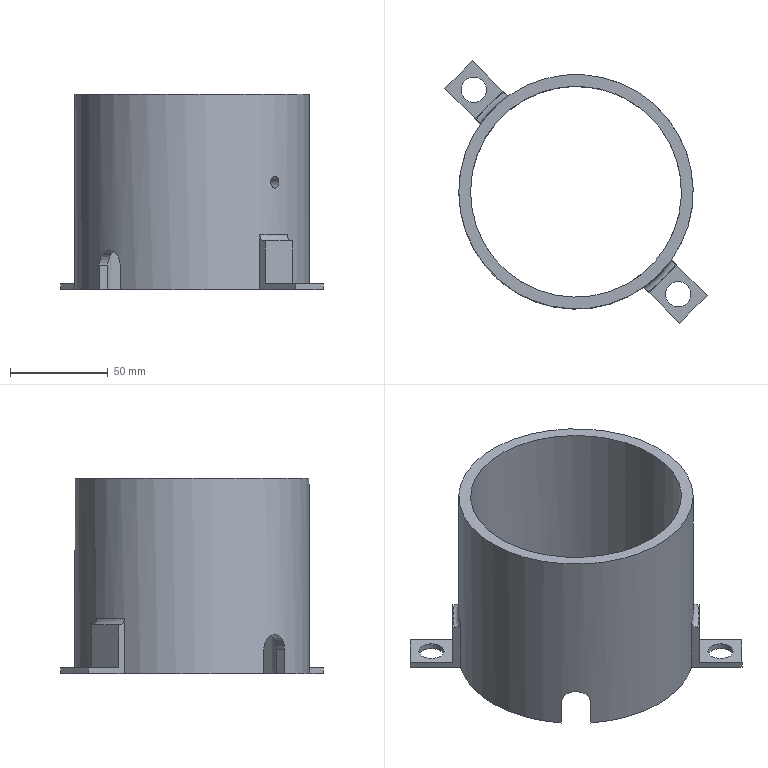Part | NX | features solid 2 | 1 solid | 30 faces | box 134.35 x 134.35 x 100 mm | volume 216597 mm3 | plane 21 | cylinder 7 | torus 2 | commonest cylinder face diameters 13 x2 15 x2 6 x1 108 x1 120 x1
STEP:
#1=CARTESIAN_POINT('',(1067.73,-417.73,-105.));
#2=VERTEX_POINT('',#1);
#3=CARTESIAN_POINT('',(1072.326,-422.326,-105.));
#4=DIRECTION('',(0.,0.,-1.));
#5=DIRECTION('',(-0.7071,0.7071,0.));
#6=AXIS2_PLACEMENT_3D('',#3,#4,#5);
#7=CIRCLE('',#6,6.5);
#8=EDGE_CURVE('',#2,#2,#7,.T.);
#9=ORIENTED_EDGE('',*,*,#8,.F.);
#10=EDGE_LOOP('',(#9));
#11=FACE_BOUND('',#10,.T.);
#12=CARTESIAN_POINT('',(1067.397,-333.21,-105.));
#13=VERTEX_POINT('',#12);
#14=CARTESIAN_POINT('',(1068.904,-404.762,-105.));
#15=VERTEX_POINT('',#14);
#16=CARTESIAN_POINT('',(1020.,-370.,-105.));
#17=DIRECTION('',(0.,0.,-1.));
#18=DIRECTION('',(-0.7071,0.7071,0.));
#19=AXIS2_PLACEMENT_3D('',#16,#17,#18);
#20=CIRCLE('',#19,60.);
#21=EDGE_CURVE('',#13,#15,#20,.T.);
#22=ORIENTED_EDGE('',*,*,#21,.T.);
#23=CARTESIAN_POINT('',(1087.175,-423.033,-105.));
#24=VERTEX_POINT('',#23);
#25=CARTESIAN_POINT('',(1065.255,-401.113,-105.));
#26=DIRECTION('',(0.7071,-0.7071,0.));
#27=VECTOR('',#26,1000.);
#28=LINE('',#25,#27);
#29=EDGE_CURVE('',#15,#24,#28,.T.);
#30=ORIENTED_EDGE('',*,*,#29,.T.);
#31=CARTESIAN_POINT('',(1073.033,-437.175,-105.));
#32=VERTEX_POINT('',#31);
#33=CARTESIAN_POINT('',(1073.033,-437.175,-105.));
#34=DIRECTION('',(0.7071,0.7071,0.));
#35=VECTOR('',#34,1000.);
#36=LINE('',#33,#35);
#37=EDGE_CURVE('',#32,#24,#36,.T.);
#38=ORIENTED_EDGE('',*,*,#37,.F.);
#39=CARTESIAN_POINT('',(1054.762,-418.904,-105.));
#40=VERTEX_POINT('',#39);
#41=CARTESIAN_POINT('',(1057.477,-421.619,-105.));
#42=DIRECTION('',(-0.7071,0.7071,0.));
#43=VECTOR('',#42,1000.);
#44=LINE('',#41,#43);
#45=EDGE_CURVE('',#32,#40,#44,.T.);
#46=ORIENTED_EDGE('',*,*,#45,.T.);
#47=CARTESIAN_POINT('',(983.21,-417.397,-105.));
#48=VERTEX_POINT('',#47);
#49=CARTESIAN_POINT('',(1020.,-370.,-105.));
#50=DIRECTION('',(0.,0.,-1.));
#51=DIRECTION('',(-0.7071,0.7071,0.));
#52=AXIS2_PLACEMENT_3D('',#49,#50,#51);
#53=CIRCLE('',#52,60.);
#54=EDGE_CURVE('',#40,#48,#53,.T.);
#55=ORIENTED_EDGE('',*,*,#54,.T.);
#56=CARTESIAN_POINT('',(987.49,-413.117,-105.));
#57=VERTEX_POINT('',#56);
#58=CARTESIAN_POINT('',(1025.303,-375.303,-105.));
#59=DIRECTION('',(-0.7071,-0.7071,0.));
#60=VECTOR('',#59,1000.);
#61=LINE('',#58,#60);
#62=EDGE_CURVE('',#57,#48,#61,.T.);
#63=ORIENTED_EDGE('',*,*,#62,.F.);
#64=CARTESIAN_POINT('',(1063.117,-337.49,-105.));
#65=VERTEX_POINT('',#64);
#66=CARTESIAN_POINT('',(1020.,-370.,-105.));
#67=DIRECTION('',(0.,0.,-1.));
#68=DIRECTION('',(-0.7071,0.7071,0.));
#69=AXIS2_PLACEMENT_3D('',#66,#67,#68);
#70=CIRCLE('',#69,54.);
#71=EDGE_CURVE('',#65,#57,#70,.T.);
#72=ORIENTED_EDGE('',*,*,#71,.F.);
#73=CARTESIAN_POINT('',(1025.303,-375.303,-105.));
#74=DIRECTION('',(-0.7071,-0.7071,0.));
#75=VECTOR('',#74,1000.);
#76=LINE('',#73,#75);
#77=EDGE_CURVE('',#13,#65,#76,.T.);
#78=ORIENTED_EDGE('',*,*,#77,.F.);
#79=EDGE_LOOP('',(#22,#30,#38,#46,#55,#63,#72,#78));
#80=FACE_BOUND('',#79,.T.);
#81=CARTESIAN_POINT('',(1020.,-370.,-105.));
#82=DIRECTION('',(0.,0.,1.));
#83=DIRECTION('',(-0.7071,0.7071,0.));
#84=AXIS2_PLACEMENT_3D('',#81,#82,#83);
#85=PLANE('',#84);
#86=ADVANCED_FACE('',(#11,#80),#85,.F.);
#87=CARTESIAN_POINT('',(982.523,-318.381,-80.));
#88=VERTEX_POINT('',#87);
#89=CARTESIAN_POINT('',(983.088,-318.946,-80.));
#90=VERTEX_POINT('',#89);
#91=CARTESIAN_POINT('',(982.523,-318.381,-80.));
#92=DIRECTION('',(0.7071,-0.7071,0.));
#93=VECTOR('',#92,1000.);
#94=LINE('',#91,#93);
#95=EDGE_CURVE('',#88,#90,#94,.T.);
#96=ORIENTED_EDGE('',*,*,#95,.F.);
#97=CARTESIAN_POINT('',(975.452,-325.452,-80.));
#98=VERTEX_POINT('',#97);
#99=CARTESIAN_POINT('',(968.381,-332.523,-80.));
#100=DIRECTION('',(0.7071,0.7071,0.));
#101=VECTOR('',#100,1000.);
#102=LINE('',#99,#101);
#103=EDGE_CURVE('',#98,#88,#102,.T.);
#104=ORIENTED_EDGE('',*,*,#103,.F.);
#105=CARTESIAN_POINT('',(1020.,-370.,-80.));
#106=DIRECTION('',(0.,0.,-1.));
#107=DIRECTION('',(-0.7071,0.7071,0.));
#108=AXIS2_PLACEMENT_3D('',#105,#106,#107);
#109=CIRCLE('',#108,63.);
#110=EDGE_CURVE('',#90,#98,#109,.F.);
#111=ORIENTED_EDGE('',*,*,#110,.F.);
#112=EDGE_LOOP('',(#96,#104,#111));
#113=FACE_BOUND('',#112,.T.);
#114=CARTESIAN_POINT('',(988.887,-324.745,-80.));
#115=DIRECTION('',(0.,0.,1.));
#116=DIRECTION('',(-0.7071,0.7071,0.));
#117=AXIS2_PLACEMENT_3D('',#114,#115,#116);
#118=PLANE('',#117);
#119=ADVANCED_FACE('',(#113),#118,.T.);
#120=CARTESIAN_POINT('',(1057.477,-421.619,-80.));
#121=VERTEX_POINT('',#120);
#122=CARTESIAN_POINT('',(1056.912,-421.054,-80.));
#123=VERTEX_POINT('',#122);
#124=CARTESIAN_POINT('',(1057.477,-421.619,-80.));
#125=DIRECTION('',(-0.7071,0.7071,0.));
#126=VECTOR('',#125,1000.);
#127=LINE('',#124,#126);
#128=EDGE_CURVE('',#121,#123,#127,.T.);
#129=ORIENTED_EDGE('',*,*,#128,.F.);
#130=CARTESIAN_POINT('',(1064.548,-414.548,-80.));
#131=VERTEX_POINT('',#130);
#132=CARTESIAN_POINT('',(1071.619,-407.477,-80.));
#133=DIRECTION('',(-0.7071,-0.7071,0.));
#134=VECTOR('',#133,1000.);
#135=LINE('',#132,#134);
#136=EDGE_CURVE('',#131,#121,#135,.T.);
#137=ORIENTED_EDGE('',*,*,#136,.F.);
#138=CARTESIAN_POINT('',(1020.,-370.,-80.));
#139=DIRECTION('',(0.,0.,-1.));
#140=DIRECTION('',(-0.7071,0.7071,0.));
#141=AXIS2_PLACEMENT_3D('',#138,#139,#140);
#142=CIRCLE('',#141,63.);
#143=EDGE_CURVE('',#123,#131,#142,.F.);
#144=ORIENTED_EDGE('',*,*,#143,.F.);
#145=EDGE_LOOP('',(#129,#137,#144));
#146=FACE_BOUND('',#145,.T.);
#147=CARTESIAN_POINT('',(1057.477,-421.619,-80.));
#148=DIRECTION('',(0.,0.,1.));
#149=DIRECTION('',(-0.7071,0.7071,0.));
#150=AXIS2_PLACEMENT_3D('',#147,#148,#149);
#151=PLANE('',#150);
#152=ADVANCED_FACE('',(#146),#151,.T.);
#153=CARTESIAN_POINT('',(1062.426,-412.426,-47.));
#154=VERTEX_POINT('',#153);
#155=CARTESIAN_POINT('',(1064.064,-410.736,-47.651));
#156=CARTESIAN_POINT('',(1062.439,-412.44,-46.675));
#157=CARTESIAN_POINT('',(1060.737,-414.062,-47.65));
#158=CARTESIAN_POINT('',(1060.01,-414.711,-49.998));
#159=CARTESIAN_POINT('',(1060.736,-414.063,-52.35));
#160=CARTESIAN_POINT('',(1062.439,-412.44,-53.324));
#161=CARTESIAN_POINT('',(1064.06,-410.74,-52.353));
#162=CARTESIAN_POINT('',(1064.711,-410.009,-50.003));
#163=CARTESIAN_POINT('',(1064.064,-410.736,-47.651));
#164=CARTESIAN_POINT('',(1062.439,-412.44,-46.675));
#165=CARTESIAN_POINT('',(1060.737,-414.062,-47.65));
#166=B_SPLINE_CURVE_WITH_KNOTS('',3,(#155,#156,#157,#158,#159,#160,#161,#162,#163,#164,#165),.UNSPECIFIED.,.T.,.F.,(1,1,1,1,1,1,1,1,1,1,1,1,1,1,1),(-0.007035,-0.00469,-0.002345,0.,0.002345,0.00469,0.007035,0.00938,0.01172,0.01407,0.01641,0.01876,0.0211,0.02345,0.02579),.UNSPECIFIED.);
#167=EDGE_CURVE('',#154,#154,#166,.T.);
#168=ORIENTED_EDGE('',*,*,#167,.F.);
#169=EDGE_LOOP('',(#168));
#170=FACE_BOUND('',#169,.T.);
#171=CARTESIAN_POINT('',(960.,-370.,-5.));
#172=VERTEX_POINT('',#171);
#173=CARTESIAN_POINT('',(1020.,-370.,-5.));
#174=DIRECTION('',(0.,0.,-1.));
#175=DIRECTION('',(-1.,0.,0.));
#176=AXIS2_PLACEMENT_3D('',#173,#174,#175);
#177=CIRCLE('',#176,60.);
#178=EDGE_CURVE('',#172,#172,#177,.T.);
#179=ORIENTED_EDGE('',*,*,#178,.T.);
#180=EDGE_LOOP('',(#179));
#181=FACE_BOUND('',#180,.T.);
#182=CARTESIAN_POINT('',(1056.79,-322.603,-92.5));
#183=VERTEX_POINT('',#182);
#184=CARTESIAN_POINT('',(1067.397,-333.21,-92.5));
#185=VERTEX_POINT('',#184);
#186=CARTESIAN_POINT('',(1056.79,-322.603,-92.5));
#187=CARTESIAN_POINT('',(1056.79,-322.603,-90.541));
#188=CARTESIAN_POINT('',(1058.106,-323.584,-86.621));
#189=CARTESIAN_POINT('',(1062.512,-327.494,-84.187));
#190=CARTESIAN_POINT('',(1066.415,-331.893,-86.633));
#191=CARTESIAN_POINT('',(1067.397,-333.21,-90.516));
#192=CARTESIAN_POINT('',(1067.397,-333.21,-92.5));
#193=B_SPLINE_CURVE_WITH_KNOTS('',3,(#186,#187,#188,#189,#190,#191,#192),.UNSPECIFIED.,.F.,.F.,(4,1,1,1,4),(0.01174,0.01761,0.02347,0.02934,0.03521),.UNSPECIFIED.);
#194=EDGE_CURVE('',#183,#185,#193,.T.);
#195=ORIENTED_EDGE('',*,*,#194,.F.);
#196=CARTESIAN_POINT('',(1056.79,-322.603,-105.));
#197=VERTEX_POINT('',#196);
#198=CARTESIAN_POINT('',(1056.79,-322.603,5.));
#199=DIRECTION('',(0.,0.,-1.));
#200=VECTOR('',#199,1000.);
#201=LINE('',#198,#200);
#202=EDGE_CURVE('',#197,#183,#201,.F.);
#203=ORIENTED_EDGE('',*,*,#202,.F.);
#204=CARTESIAN_POINT('',(985.238,-321.096,-105.));
#205=VERTEX_POINT('',#204);
#206=CARTESIAN_POINT('',(1020.,-370.,-105.));
#207=DIRECTION('',(0.,0.,-1.));
#208=DIRECTION('',(-0.7071,0.7071,0.));
#209=AXIS2_PLACEMENT_3D('',#206,#207,#208);
#210=CIRCLE('',#209,60.);
#211=EDGE_CURVE('',#205,#197,#210,.T.);
#212=ORIENTED_EDGE('',*,*,#211,.F.);
#213=CARTESIAN_POINT('',(985.238,-321.096,-77.));
#214=VERTEX_POINT('',#213);
#215=CARTESIAN_POINT('',(985.238,-321.096,5.));
#216=DIRECTION('',(0.,0.,-1.));
#217=VECTOR('',#216,1000.);
#218=LINE('',#215,#217);
#219=EDGE_CURVE('',#205,#214,#218,.F.);
#220=ORIENTED_EDGE('',*,*,#219,.T.);
#221=CARTESIAN_POINT('',(971.096,-335.238,-77.));
#222=VERTEX_POINT('',#221);
#223=CARTESIAN_POINT('',(1020.,-370.,-77.));
#224=DIRECTION('',(0.,0.,-1.));
#225=DIRECTION('',(-0.7071,0.7071,0.));
#226=AXIS2_PLACEMENT_3D('',#223,#224,#225);
#227=CIRCLE('',#226,60.);
#228=EDGE_CURVE('',#222,#214,#227,.T.);
#229=ORIENTED_EDGE('',*,*,#228,.F.);
#230=CARTESIAN_POINT('',(971.096,-335.238,-105.));
#231=VERTEX_POINT('',#230);
#232=CARTESIAN_POINT('',(971.096,-335.238,5.));
#233=DIRECTION('',(0.,0.,-1.));
#234=VECTOR('',#233,1000.);
#235=LINE('',#232,#234);
#236=EDGE_CURVE('',#222,#231,#235,.T.);
#237=ORIENTED_EDGE('',*,*,#236,.T.);
#238=CARTESIAN_POINT('',(972.603,-406.79,-105.));
#239=VERTEX_POINT('',#238);
#240=CARTESIAN_POINT('',(1020.,-370.,-105.));
#241=DIRECTION('',(0.,0.,-1.));
#242=DIRECTION('',(-0.7071,0.7071,0.));
#243=AXIS2_PLACEMENT_3D('',#240,#241,#242);
#244=CIRCLE('',#243,60.);
#245=EDGE_CURVE('',#239,#231,#244,.T.);
#246=ORIENTED_EDGE('',*,*,#245,.F.);
#247=CARTESIAN_POINT('',(972.603,-406.79,-92.5));
#248=VERTEX_POINT('',#247);
#249=CARTESIAN_POINT('',(972.603,-406.79,5.));
#250=DIRECTION('',(0.,0.,-1.));
#251=VECTOR('',#250,1000.);
#252=LINE('',#249,#251);
#253=EDGE_CURVE('',#248,#239,#252,.T.);
#254=ORIENTED_EDGE('',*,*,#253,.F.);
#255=CARTESIAN_POINT('',(983.21,-417.397,-92.5));
#256=VERTEX_POINT('',#255);
#257=CARTESIAN_POINT('',(983.21,-417.397,-92.5));
#258=CARTESIAN_POINT('',(983.21,-417.397,-90.517));
#259=CARTESIAN_POINT('',(981.896,-416.418,-86.634));
#260=CARTESIAN_POINT('',(977.485,-412.504,-84.184));
#261=CARTESIAN_POINT('',(973.581,-408.101,-86.631));
#262=CARTESIAN_POINT('',(972.603,-406.79,-90.542));
#263=CARTESIAN_POINT('',(972.603,-406.79,-92.5));
#264=B_SPLINE_CURVE_WITH_KNOTS('',3,(#257,#258,#259,#260,#261,#262,#263),.UNSPECIFIED.,.F.,.F.,(4,1,1,1,4),(0.03521,0.04108,0.04694,0.05281,0.05868),.UNSPECIFIED.);
#265=EDGE_CURVE('',#256,#248,#264,.T.);
#266=ORIENTED_EDGE('',*,*,#265,.F.);
#267=CARTESIAN_POINT('',(983.21,-417.397,5.));
#268=DIRECTION('',(0.,0.,-1.));
#269=VECTOR('',#268,1000.);
#270=LINE('',#267,#269);
#271=EDGE_CURVE('',#48,#256,#270,.F.);
#272=ORIENTED_EDGE('',*,*,#271,.F.);
#273=ORIENTED_EDGE('',*,*,#54,.F.);
#274=CARTESIAN_POINT('',(1054.762,-418.904,-77.));
#275=VERTEX_POINT('',#274);
#276=CARTESIAN_POINT('',(1054.762,-418.904,5.));
#277=DIRECTION('',(0.,0.,-1.));
#278=VECTOR('',#277,1000.);
#279=LINE('',#276,#278);
#280=EDGE_CURVE('',#40,#275,#279,.F.);
#281=ORIENTED_EDGE('',*,*,#280,.T.);
#282=CARTESIAN_POINT('',(1068.904,-404.762,-77.));
#283=VERTEX_POINT('',#282);
#284=CARTESIAN_POINT('',(1020.,-370.,-77.));
#285=DIRECTION('',(0.,0.,-1.));
#286=DIRECTION('',(-0.7071,0.7071,0.));
#287=AXIS2_PLACEMENT_3D('',#284,#285,#286);
#288=CIRCLE('',#287,60.);
#289=EDGE_CURVE('',#283,#275,#288,.T.);
#290=ORIENTED_EDGE('',*,*,#289,.F.);
#291=CARTESIAN_POINT('',(1068.904,-404.762,5.));
#292=DIRECTION('',(0.,0.,-1.));
#293=VECTOR('',#292,1000.);
#294=LINE('',#291,#293);
#295=EDGE_CURVE('',#283,#15,#294,.T.);
#296=ORIENTED_EDGE('',*,*,#295,.T.);
#297=ORIENTED_EDGE('',*,*,#21,.F.);
#298=CARTESIAN_POINT('',(1067.397,-333.21,5.));
#299=DIRECTION('',(0.,0.,-1.));
#300=VECTOR('',#299,1000.);
#301=LINE('',#298,#300);
#302=EDGE_CURVE('',#185,#13,#301,.T.);
#303=ORIENTED_EDGE('',*,*,#302,.F.);
#304=EDGE_LOOP('',(#195,#203,#212,#220,#229,#237,#246,#254,#266,#272,#273,#281,#290,#296,#297,#303));
#305=FACE_BOUND('',#304,.T.);
#306=CARTESIAN_POINT('',(1020.,-370.,5.));
#307=DIRECTION('',(0.,0.,-1.));
#308=DIRECTION('',(0.7071,-0.7071,0.));
#309=AXIS2_PLACEMENT_3D('',#306,#307,#308);
#310=CYLINDRICAL_SURFACE('',#309,60.);
#311=ADVANCED_FACE('',(#170,#181,#305),#310,.T.);
#312=CARTESIAN_POINT('',(1063.117,-337.49,-92.5));
#313=VERTEX_POINT('',#312);
#314=CARTESIAN_POINT('',(1063.117,-337.49,5.));
#315=DIRECTION('',(0.,0.,-1.));
#316=VECTOR('',#315,1000.);
#317=LINE('',#314,#316);
#318=EDGE_CURVE('',#313,#65,#317,.T.);
#319=ORIENTED_EDGE('',*,*,#318,.T.);
#320=ORIENTED_EDGE('',*,*,#71,.T.);
#321=CARTESIAN_POINT('',(987.49,-413.117,-92.5));
#322=VERTEX_POINT('',#321);
#323=CARTESIAN_POINT('',(987.49,-413.117,5.));
#324=DIRECTION('',(0.,0.,-1.));
#325=VECTOR('',#324,1000.);
#326=LINE('',#323,#325);
#327=EDGE_CURVE('',#57,#322,#326,.F.);
#328=ORIENTED_EDGE('',*,*,#327,.T.);
#329=CARTESIAN_POINT('',(976.883,-402.51,-92.5));
#330=VERTEX_POINT('',#329);
#331=CARTESIAN_POINT('',(987.49,-413.117,-92.5));
#332=CARTESIAN_POINT('',(987.49,-413.117,-90.517));
#333=CARTESIAN_POINT('',(986.158,-412.157,-86.634));
#334=CARTESIAN_POINT('',(981.719,-408.271,-84.184));
#335=CARTESIAN_POINT('',(977.842,-403.84,-86.631));
#336=CARTESIAN_POINT('',(976.883,-402.51,-90.541));
#337=CARTESIAN_POINT('',(976.883,-402.51,-92.5));
#338=B_SPLINE_CURVE_WITH_KNOTS('',3,(#331,#332,#333,#334,#335,#336,#337),.UNSPECIFIED.,.F.,.F.,(4,1,1,1,4),(0.03522,0.04109,0.04695,0.05282,0.05869),.UNSPECIFIED.);
#339=EDGE_CURVE('',#322,#330,#338,.T.);
#340=ORIENTED_EDGE('',*,*,#339,.T.);
#341=CARTESIAN_POINT('',(976.883,-402.51,-105.));
#342=VERTEX_POINT('',#341);
#343=CARTESIAN_POINT('',(976.883,-402.51,5.));
#344=DIRECTION('',(0.,0.,-1.));
#345=VECTOR('',#344,1000.);
#346=LINE('',#343,#345);
#347=EDGE_CURVE('',#330,#342,#346,.T.);
#348=ORIENTED_EDGE('',*,*,#347,.T.);
#349=CARTESIAN_POINT('',(1052.51,-326.883,-105.));
#350=VERTEX_POINT('',#349);
#351=CARTESIAN_POINT('',(1020.,-370.,-105.));
#352=DIRECTION('',(0.,0.,-1.));
#353=DIRECTION('',(-0.7071,0.7071,0.));
#354=AXIS2_PLACEMENT_3D('',#351,#352,#353);
#355=CIRCLE('',#354,54.);
#356=EDGE_CURVE('',#342,#350,#355,.T.);
#357=ORIENTED_EDGE('',*,*,#356,.T.);
#358=CARTESIAN_POINT('',(1052.51,-326.883,-92.5));
#359=VERTEX_POINT('',#358);
#360=CARTESIAN_POINT('',(1052.51,-326.883,5.));
#361=DIRECTION('',(0.,0.,-1.));
#362=VECTOR('',#361,1000.);
#363=LINE('',#360,#362);
#364=EDGE_CURVE('',#350,#359,#363,.F.);
#365=ORIENTED_EDGE('',*,*,#364,.T.);
#366=CARTESIAN_POINT('',(1052.51,-326.883,-92.5));
#367=CARTESIAN_POINT('',(1052.51,-326.883,-90.541));
#368=CARTESIAN_POINT('',(1053.845,-327.845,-86.621));
#369=CARTESIAN_POINT('',(1058.279,-331.727,-84.187));
#370=CARTESIAN_POINT('',(1062.154,-336.154,-86.632));
#371=CARTESIAN_POINT('',(1063.117,-337.49,-90.517));
#372=CARTESIAN_POINT('',(1063.117,-337.49,-92.5));
#373=B_SPLINE_CURVE_WITH_KNOTS('',3,(#366,#367,#368,#369,#370,#371,#372),.UNSPECIFIED.,.F.,.F.,(4,1,1,1,4),(0.01174,0.01761,0.02348,0.02935,0.03522),.UNSPECIFIED.);
#374=EDGE_CURVE('',#359,#313,#373,.T.);
#375=ORIENTED_EDGE('',*,*,#374,.T.);
#376=EDGE_LOOP('',(#319,#320,#328,#340,#348,#357,#365,#375));
#377=FACE_BOUND('',#376,.T.);
#378=CARTESIAN_POINT('',(1058.184,-408.184,-47.));
#379=VERTEX_POINT('',#378);
#380=CARTESIAN_POINT('',(1059.818,-406.49,-47.651));
#381=CARTESIAN_POINT('',(1058.198,-408.199,-46.675));
#382=CARTESIAN_POINT('',(1056.492,-409.817,-47.65));
#383=CARTESIAN_POINT('',(1055.76,-410.461,-49.998));
#384=CARTESIAN_POINT('',(1056.491,-409.818,-52.35));
#385=CARTESIAN_POINT('',(1058.198,-408.199,-53.324));
#386=CARTESIAN_POINT('',(1059.815,-406.494,-52.353));
#387=CARTESIAN_POINT('',(1060.461,-405.759,-50.003));
#388=CARTESIAN_POINT('',(1059.818,-406.49,-47.651));
#389=CARTESIAN_POINT('',(1058.198,-408.199,-46.675));
#390=CARTESIAN_POINT('',(1056.492,-409.817,-47.65));
#391=B_SPLINE_CURVE_WITH_KNOTS('',3,(#380,#381,#382,#383,#384,#385,#386,#387,#388,#389,#390),.UNSPECIFIED.,.T.,.F.,(1,1,1,1,1,1,1,1,1,1,1,1,1,1,1),(-0.007035,-0.00469,-0.002345,0.,0.002345,0.00469,0.007035,0.00938,0.01173,0.01407,0.01642,0.01876,0.02111,0.02345,0.0258),.UNSPECIFIED.);
#392=EDGE_CURVE('',#379,#379,#391,.T.);
#393=ORIENTED_EDGE('',*,*,#392,.T.);
#394=EDGE_LOOP('',(#393));
#395=FACE_BOUND('',#394,.T.);
#396=CARTESIAN_POINT('',(966.,-370.,-5.));
#397=VERTEX_POINT('',#396);
#398=CARTESIAN_POINT('',(1020.,-370.,-5.));
#399=DIRECTION('',(0.,0.,-1.));
#400=DIRECTION('',(-1.,0.,0.));
#401=AXIS2_PLACEMENT_3D('',#398,#399,#400);
#402=CIRCLE('',#401,54.);
#403=EDGE_CURVE('',#397,#397,#402,.T.);
#404=ORIENTED_EDGE('',*,*,#403,.F.);
#405=EDGE_LOOP('',(#404));
#406=FACE_BOUND('',#405,.T.);
#407=CARTESIAN_POINT('',(1020.,-370.,5.));
#408=DIRECTION('',(0.,0.,-1.));
#409=DIRECTION('',(0.7071,-0.7071,0.));
#410=AXIS2_PLACEMENT_3D('',#407,#408,#409);
#411=CYLINDRICAL_SURFACE('',#410,54.);
#412=ADVANCED_FACE('',(#377,#395,#406),#411,.F.);
#413=ORIENTED_EDGE('',*,*,#403,.T.);
#414=EDGE_LOOP('',(#413));
#415=FACE_BOUND('',#414,.T.);
#416=ORIENTED_EDGE('',*,*,#178,.F.);
#417=EDGE_LOOP('',(#416));
#418=FACE_BOUND('',#417,.T.);
#419=CARTESIAN_POINT('',(1020.,-370.,-5.));
#420=DIRECTION('',(0.,0.,1.));
#421=DIRECTION('',(-0.7071,0.7071,0.));
#422=AXIS2_PLACEMENT_3D('',#419,#420,#421);
#423=PLANE('',#422);
#424=ADVANCED_FACE('',(#415,#418),#423,.T.);
#425=ORIENTED_EDGE('',*,*,#356,.F.);
#426=CARTESIAN_POINT('',(1014.697,-364.697,-105.));
#427=DIRECTION('',(0.7071,0.7071,0.));
#428=VECTOR('',#427,1000.);
#429=LINE('',#426,#428);
#430=EDGE_CURVE('',#239,#342,#429,.T.);
#431=ORIENTED_EDGE('',*,*,#430,.F.);
#432=ORIENTED_EDGE('',*,*,#245,.T.);
#433=CARTESIAN_POINT('',(952.825,-316.967,-105.));
#434=VERTEX_POINT('',#433);
#435=CARTESIAN_POINT('',(974.745,-338.887,-105.));
#436=DIRECTION('',(-0.7071,0.7071,0.));
#437=VECTOR('',#436,1000.);
#438=LINE('',#435,#437);
#439=EDGE_CURVE('',#231,#434,#438,.T.);
#440=ORIENTED_EDGE('',*,*,#439,.T.);
#441=CARTESIAN_POINT('',(966.967,-302.825,-105.));
#442=VERTEX_POINT('',#441);
#443=CARTESIAN_POINT('',(966.967,-302.825,-105.));
#444=DIRECTION('',(-0.7071,-0.7071,0.));
#445=VECTOR('',#444,1000.);
#446=LINE('',#443,#445);
#447=EDGE_CURVE('',#442,#434,#446,.T.);
#448=ORIENTED_EDGE('',*,*,#447,.F.);
#449=CARTESIAN_POINT('',(982.523,-318.381,-105.));
#450=DIRECTION('',(0.7071,-0.7071,0.));
#451=VECTOR('',#450,1000.);
#452=LINE('',#449,#451);
#453=EDGE_CURVE('',#442,#205,#452,.T.);
#454=ORIENTED_EDGE('',*,*,#453,.T.);
#455=ORIENTED_EDGE('',*,*,#211,.T.);
#456=CARTESIAN_POINT('',(1014.697,-364.697,-105.));
#457=DIRECTION('',(0.7071,0.7071,0.));
#458=VECTOR('',#457,1000.);
#459=LINE('',#456,#458);
#460=EDGE_CURVE('',#350,#197,#459,.T.);
#461=ORIENTED_EDGE('',*,*,#460,.F.);
#462=EDGE_LOOP('',(#425,#431,#432,#440,#448,#454,#455,#461));
#463=FACE_BOUND('',#462,.T.);
#464=CARTESIAN_POINT('',(963.078,-313.078,-105.));
#465=VERTEX_POINT('',#464);
#466=CARTESIAN_POINT('',(967.674,-317.674,-105.));
#467=DIRECTION('',(0.,0.,-1.));
#468=DIRECTION('',(-0.7071,0.7071,0.));
#469=AXIS2_PLACEMENT_3D('',#466,#467,#468);
#470=CIRCLE('',#469,6.5);
#471=EDGE_CURVE('',#465,#465,#470,.T.);
#472=ORIENTED_EDGE('',*,*,#471,.F.);
#473=EDGE_LOOP('',(#472));
#474=FACE_BOUND('',#473,.T.);
#475=CARTESIAN_POINT('',(1020.,-370.,-105.));
#476=DIRECTION('',(0.,0.,1.));
#477=DIRECTION('',(-0.7071,0.7071,0.));
#478=AXIS2_PLACEMENT_3D('',#475,#476,#477);
#479=PLANE('',#478);
#480=ADVANCED_FACE('',(#463,#474),#479,.F.);
#481=CARTESIAN_POINT('',(1071.619,-407.477,-80.));
#482=VERTEX_POINT('',#481);
#483=CARTESIAN_POINT('',(1071.619,-407.477,-80.));
#484=DIRECTION('',(-0.7071,-0.7071,0.));
#485=VECTOR('',#484,1000.);
#486=LINE('',#483,#485);
#487=EDGE_CURVE('',#482,#131,#486,.T.);
#488=ORIENTED_EDGE('',*,*,#487,.F.);
#489=CARTESIAN_POINT('',(1071.054,-406.912,-80.));
#490=VERTEX_POINT('',#489);
#491=CARTESIAN_POINT('',(1065.255,-401.113,-80.));
#492=DIRECTION('',(0.7071,-0.7071,0.));
#493=VECTOR('',#492,1000.);
#494=LINE('',#491,#493);
#495=EDGE_CURVE('',#490,#482,#494,.T.);
#496=ORIENTED_EDGE('',*,*,#495,.F.);
#497=CARTESIAN_POINT('',(1020.,-370.,-80.));
#498=DIRECTION('',(0.,0.,-1.));
#499=DIRECTION('',(-0.7071,0.7071,0.));
#500=AXIS2_PLACEMENT_3D('',#497,#498,#499);
#501=CIRCLE('',#500,63.);
#502=EDGE_CURVE('',#131,#490,#501,.F.);
#503=ORIENTED_EDGE('',*,*,#502,.F.);
#504=EDGE_LOOP('',(#488,#496,#503));
#505=FACE_BOUND('',#504,.T.);
#506=CARTESIAN_POINT('',(1057.477,-421.619,-80.));
#507=DIRECTION('',(0.,0.,1.));
#508=DIRECTION('',(-0.7071,0.7071,0.));
#509=AXIS2_PLACEMENT_3D('',#506,#507,#508);
#510=PLANE('',#509);
#511=ADVANCED_FACE('',(#505),#510,.T.);
#512=ORIENTED_EDGE('',*,*,#45,.F.);
#513=CARTESIAN_POINT('',(1073.033,-437.175,-102.));
#514=VERTEX_POINT('',#513);
#515=CARTESIAN_POINT('',(1073.033,-437.175,-102.));
#516=DIRECTION('',(0.,0.,-1.));
#517=VECTOR('',#516,1000.);
#518=LINE('',#515,#517);
#519=EDGE_CURVE('',#514,#32,#518,.T.);
#520=ORIENTED_EDGE('',*,*,#519,.F.);
#521=CARTESIAN_POINT('',(1057.477,-421.619,-102.));
#522=VERTEX_POINT('',#521);
#523=CARTESIAN_POINT('',(1057.477,-421.619,-102.));
#524=DIRECTION('',(0.7071,-0.7071,0.));
#525=VECTOR('',#524,1000.);
#526=LINE('',#523,#525);
#527=EDGE_CURVE('',#522,#514,#526,.T.);
#528=ORIENTED_EDGE('',*,*,#527,.F.);
#529=CARTESIAN_POINT('',(1057.477,-421.619,-80.));
#530=DIRECTION('',(0.,0.,-1.));
#531=VECTOR('',#530,1000.);
#532=LINE('',#529,#531);
#533=EDGE_CURVE('',#121,#522,#532,.T.);
#534=ORIENTED_EDGE('',*,*,#533,.F.);
#535=ORIENTED_EDGE('',*,*,#128,.T.);
#536=CARTESIAN_POINT('',(1054.762,-418.904,-77.));
#537=CARTESIAN_POINT('',(1054.762,-418.904,-77.798));
#538=CARTESIAN_POINT('',(1055.238,-419.38,-79.356));
#539=CARTESIAN_POINT('',(1056.348,-420.49,-80.));
#540=CARTESIAN_POINT('',(1056.912,-421.054,-80.));
#541=B_SPLINE_CURVE_WITH_KNOTS('',3,(#536,#537,#538,#539,#540),.UNSPECIFIED.,.F.,.F.,(4,1,4),(0.,0.002359,0.004718),.UNSPECIFIED.);
#542=EDGE_CURVE('',#275,#123,#541,.T.);
#543=ORIENTED_EDGE('',*,*,#542,.F.);
#544=ORIENTED_EDGE('',*,*,#280,.F.);
#545=EDGE_LOOP('',(#512,#520,#528,#534,#535,#543,#544));
#546=FACE_BOUND('',#545,.T.);
#547=CARTESIAN_POINT('',(1057.477,-421.619,-80.));
#548=DIRECTION('',(0.7071,0.7071,0.));
#549=DIRECTION('',(0.7071,-0.7071,0.));
#550=AXIS2_PLACEMENT_3D('',#547,#548,#549);
#551=PLANE('',#550);
#552=ADVANCED_FACE('',(#546),#551,.F.);
#553=ORIENTED_EDGE('',*,*,#495,.T.);
#554=CARTESIAN_POINT('',(1071.619,-407.477,-102.));
#555=VERTEX_POINT('',#554);
#556=CARTESIAN_POINT('',(1071.619,-407.477,-80.));
#557=DIRECTION('',(0.,0.,-1.));
#558=VECTOR('',#557,1000.);
#559=LINE('',#556,#558);
#560=EDGE_CURVE('',#482,#555,#559,.T.);
#561=ORIENTED_EDGE('',*,*,#560,.T.);
#562=CARTESIAN_POINT('',(1087.175,-423.033,-102.));
#563=VERTEX_POINT('',#562);
#564=CARTESIAN_POINT('',(1087.175,-423.033,-102.));
#565=DIRECTION('',(-0.7071,0.7071,0.));
#566=VECTOR('',#565,1000.);
#567=LINE('',#564,#566);
#568=EDGE_CURVE('',#563,#555,#567,.T.);
#569=ORIENTED_EDGE('',*,*,#568,.F.);
#570=CARTESIAN_POINT('',(1087.175,-423.033,-102.));
#571=DIRECTION('',(0.,0.,-1.));
#572=VECTOR('',#571,1000.);
#573=LINE('',#570,#572);
#574=EDGE_CURVE('',#563,#24,#573,.T.);
#575=ORIENTED_EDGE('',*,*,#574,.T.);
#576=ORIENTED_EDGE('',*,*,#29,.F.);
#577=ORIENTED_EDGE('',*,*,#295,.F.);
#578=CARTESIAN_POINT('',(1071.054,-406.912,-80.));
#579=CARTESIAN_POINT('',(1070.49,-406.348,-80.));
#580=CARTESIAN_POINT('',(1069.382,-405.24,-79.359));
#581=CARTESIAN_POINT('',(1068.904,-404.762,-77.798));
#582=CARTESIAN_POINT('',(1068.904,-404.762,-77.));
#583=B_SPLINE_CURVE_WITH_KNOTS('',3,(#578,#579,#580,#581,#582),.UNSPECIFIED.,.F.,.F.,(4,1,4),(0.,0.002359,0.004718),.UNSPECIFIED.);
#584=EDGE_CURVE('',#490,#283,#583,.T.);
#585=ORIENTED_EDGE('',*,*,#584,.F.);
#586=EDGE_LOOP('',(#553,#561,#569,#575,#576,#577,#585));
#587=FACE_BOUND('',#586,.T.);
#588=CARTESIAN_POINT('',(1065.255,-401.113,-80.));
#589=DIRECTION('',(-0.7071,-0.7071,0.));
#590=DIRECTION('',(-0.7071,0.7071,0.));
#591=AXIS2_PLACEMENT_3D('',#588,#589,#590);
#592=PLANE('',#591);
#593=ADVANCED_FACE('',(#587),#592,.F.);
#594=ORIENTED_EDGE('',*,*,#560,.F.);
#595=ORIENTED_EDGE('',*,*,#487,.T.);
#596=ORIENTED_EDGE('',*,*,#136,.T.);
#597=ORIENTED_EDGE('',*,*,#533,.T.);
#598=CARTESIAN_POINT('',(1071.619,-407.477,-102.));
#599=DIRECTION('',(-0.7071,-0.7071,0.));
#600=VECTOR('',#599,1000.);
#601=LINE('',#598,#600);
#602=EDGE_CURVE('',#555,#522,#601,.T.);
#603=ORIENTED_EDGE('',*,*,#602,.F.);
#604=EDGE_LOOP('',(#594,#595,#596,#597,#603));
#605=FACE_BOUND('',#604,.T.);
#606=CARTESIAN_POINT('',(1071.619,-407.477,-80.));
#607=DIRECTION('',(-0.7071,0.7071,0.));
#608=DIRECTION('',(0.,0.,-1.));
#609=AXIS2_PLACEMENT_3D('',#606,#607,#608);
#610=PLANE('',#609);
#611=ADVANCED_FACE('',(#605),#610,.F.);
#612=CARTESIAN_POINT('',(968.381,-332.523,-80.));
#613=VERTEX_POINT('',#612);
#614=CARTESIAN_POINT('',(968.381,-332.523,-80.));
#615=DIRECTION('',(0.7071,0.7071,0.));
#616=VECTOR('',#615,1000.);
#617=LINE('',#614,#616);
#618=EDGE_CURVE('',#613,#98,#617,.T.);
#619=ORIENTED_EDGE('',*,*,#618,.F.);
#620=CARTESIAN_POINT('',(968.946,-333.088,-80.));
#621=VERTEX_POINT('',#620);
#622=CARTESIAN_POINT('',(974.745,-338.887,-80.));
#623=DIRECTION('',(-0.7071,0.7071,0.));
#624=VECTOR('',#623,1000.);
#625=LINE('',#622,#624);
#626=EDGE_CURVE('',#621,#613,#625,.T.);
#627=ORIENTED_EDGE('',*,*,#626,.F.);
#628=CARTESIAN_POINT('',(1020.,-370.,-80.));
#629=DIRECTION('',(0.,0.,-1.));
#630=DIRECTION('',(-0.7071,0.7071,0.));
#631=AXIS2_PLACEMENT_3D('',#628,#629,#630);
#632=CIRCLE('',#631,63.);
#633=EDGE_CURVE('',#98,#621,#632,.F.);
#634=ORIENTED_EDGE('',*,*,#633,.F.);
#635=EDGE_LOOP('',(#619,#627,#634));
#636=FACE_BOUND('',#635,.T.);
#637=CARTESIAN_POINT('',(988.887,-324.745,-80.));
#638=DIRECTION('',(0.,0.,1.));
#639=DIRECTION('',(-0.7071,0.7071,0.));
#640=AXIS2_PLACEMENT_3D('',#637,#638,#639);
#641=PLANE('',#640);
#642=ADVANCED_FACE('',(#636),#641,.T.);
#643=ORIENTED_EDGE('',*,*,#453,.F.);
#644=CARTESIAN_POINT('',(966.967,-302.825,-102.));
#645=VERTEX_POINT('',#644);
#646=CARTESIAN_POINT('',(966.967,-302.825,-102.));
#647=DIRECTION('',(0.,0.,-1.));
#648=VECTOR('',#647,1000.);
#649=LINE('',#646,#648);
#650=EDGE_CURVE('',#645,#442,#649,.T.);
#651=ORIENTED_EDGE('',*,*,#650,.F.);
#652=CARTESIAN_POINT('',(982.523,-318.381,-102.));
#653=VERTEX_POINT('',#652);
#654=CARTESIAN_POINT('',(982.523,-318.381,-102.));
#655=DIRECTION('',(-0.7071,0.7071,0.));
#656=VECTOR('',#655,1000.);
#657=LINE('',#654,#656);
#658=EDGE_CURVE('',#653,#645,#657,.T.);
#659=ORIENTED_EDGE('',*,*,#658,.F.);
#660=CARTESIAN_POINT('',(982.523,-318.381,-80.));
#661=DIRECTION('',(0.,0.,-1.));
#662=VECTOR('',#661,1000.);
#663=LINE('',#660,#662);
#664=EDGE_CURVE('',#88,#653,#663,.T.);
#665=ORIENTED_EDGE('',*,*,#664,.F.);
#666=ORIENTED_EDGE('',*,*,#95,.T.);
#667=CARTESIAN_POINT('',(985.238,-321.096,-77.));
#668=CARTESIAN_POINT('',(985.238,-321.096,-77.798));
#669=CARTESIAN_POINT('',(984.762,-320.62,-79.356));
#670=CARTESIAN_POINT('',(983.652,-319.51,-80.));
#671=CARTESIAN_POINT('',(983.088,-318.946,-80.));
#672=B_SPLINE_CURVE_WITH_KNOTS('',3,(#667,#668,#669,#670,#671),.UNSPECIFIED.,.F.,.F.,(4,1,4),(0.,0.002359,0.004718),.UNSPECIFIED.);
#673=EDGE_CURVE('',#214,#90,#672,.T.);
#674=ORIENTED_EDGE('',*,*,#673,.F.);
#675=ORIENTED_EDGE('',*,*,#219,.F.);
#676=EDGE_LOOP('',(#643,#651,#659,#665,#666,#674,#675));
#677=FACE_BOUND('',#676,.T.);
#678=CARTESIAN_POINT('',(982.523,-318.381,-80.));
#679=DIRECTION('',(-0.7071,-0.7071,0.));
#680=DIRECTION('',(-0.7071,0.7071,0.));
#681=AXIS2_PLACEMENT_3D('',#678,#679,#680);
#682=PLANE('',#681);
#683=ADVANCED_FACE('',(#677),#682,.F.);
#684=ORIENTED_EDGE('',*,*,#626,.T.);
#685=CARTESIAN_POINT('',(968.381,-332.523,-102.));
#686=VERTEX_POINT('',#685);
#687=CARTESIAN_POINT('',(968.381,-332.523,-80.));
#688=DIRECTION('',(0.,0.,-1.));
#689=VECTOR('',#688,1000.);
#690=LINE('',#687,#689);
#691=EDGE_CURVE('',#613,#686,#690,.T.);
#692=ORIENTED_EDGE('',*,*,#691,.T.);
#693=CARTESIAN_POINT('',(952.825,-316.967,-102.));
#694=VERTEX_POINT('',#693);
#695=CARTESIAN_POINT('',(952.825,-316.967,-102.));
#696=DIRECTION('',(0.7071,-0.7071,0.));
#697=VECTOR('',#696,1000.);
#698=LINE('',#695,#697);
#699=EDGE_CURVE('',#694,#686,#698,.T.);
#700=ORIENTED_EDGE('',*,*,#699,.F.);
#701=CARTESIAN_POINT('',(952.825,-316.967,-102.));
#702=DIRECTION('',(0.,0.,-1.));
#703=VECTOR('',#702,1000.);
#704=LINE('',#701,#703);
#705=EDGE_CURVE('',#694,#434,#704,.T.);
#706=ORIENTED_EDGE('',*,*,#705,.T.);
#707=ORIENTED_EDGE('',*,*,#439,.F.);
#708=ORIENTED_EDGE('',*,*,#236,.F.);
#709=CARTESIAN_POINT('',(968.946,-333.088,-80.));
#710=CARTESIAN_POINT('',(969.51,-333.652,-80.));
#711=CARTESIAN_POINT('',(970.618,-334.76,-79.359));
#712=CARTESIAN_POINT('',(971.096,-335.238,-77.798));
#713=CARTESIAN_POINT('',(971.096,-335.238,-77.));
#714=B_SPLINE_CURVE_WITH_KNOTS('',3,(#709,#710,#711,#712,#713),.UNSPECIFIED.,.F.,.F.,(4,1,4),(0.,0.002359,0.004718),.UNSPECIFIED.);
#715=EDGE_CURVE('',#621,#222,#714,.T.);
#716=ORIENTED_EDGE('',*,*,#715,.F.);
#717=EDGE_LOOP('',(#684,#692,#700,#706,#707,#708,#716));
#718=FACE_BOUND('',#717,.T.);
#719=CARTESIAN_POINT('',(974.745,-338.887,-80.));
#720=DIRECTION('',(0.7071,0.7071,0.));
#721=DIRECTION('',(0.,0.,1.));
#722=AXIS2_PLACEMENT_3D('',#719,#720,#721);
#723=PLANE('',#722);
#724=ADVANCED_FACE('',(#718),#723,.F.);
#725=ORIENTED_EDGE('',*,*,#691,.F.);
#726=ORIENTED_EDGE('',*,*,#618,.T.);
#727=ORIENTED_EDGE('',*,*,#103,.T.);
#728=ORIENTED_EDGE('',*,*,#664,.T.);
#729=CARTESIAN_POINT('',(968.381,-332.523,-102.));
#730=DIRECTION('',(0.7071,0.7071,0.));
#731=VECTOR('',#730,1000.);
#732=LINE('',#729,#731);
#733=EDGE_CURVE('',#686,#653,#732,.T.);
#734=ORIENTED_EDGE('',*,*,#733,.F.);
#735=EDGE_LOOP('',(#725,#726,#727,#728,#734));
#736=FACE_BOUND('',#735,.T.);
#737=CARTESIAN_POINT('',(968.381,-332.523,-80.));
#738=DIRECTION('',(0.7071,-0.7071,0.));
#739=DIRECTION('',(0.,0.,1.));
#740=AXIS2_PLACEMENT_3D('',#737,#738,#739);
#741=PLANE('',#740);
#742=ADVANCED_FACE('',(#736),#741,.F.);
#743=ORIENTED_EDGE('',*,*,#447,.T.);
#744=ORIENTED_EDGE('',*,*,#705,.F.);
#745=CARTESIAN_POINT('',(966.967,-302.825,-102.));
#746=DIRECTION('',(-0.7071,-0.7071,0.));
#747=VECTOR('',#746,1000.);
#748=LINE('',#745,#747);
#749=EDGE_CURVE('',#645,#694,#748,.T.);
#750=ORIENTED_EDGE('',*,*,#749,.F.);
#751=ORIENTED_EDGE('',*,*,#650,.T.);
#752=EDGE_LOOP('',(#743,#744,#750,#751));
#753=FACE_BOUND('',#752,.T.);
#754=CARTESIAN_POINT('',(966.967,-302.825,-102.));
#755=DIRECTION('',(-0.7071,0.7071,0.));
#756=DIRECTION('',(0.,0.,-1.));
#757=AXIS2_PLACEMENT_3D('',#754,#755,#756);
#758=PLANE('',#757);
#759=ADVANCED_FACE('',(#753),#758,.T.);
#760=CARTESIAN_POINT('',(963.078,-313.078,-102.));
#761=VERTEX_POINT('',#760);
#762=CARTESIAN_POINT('',(967.674,-317.674,-102.));
#763=DIRECTION('',(0.,0.,-1.));
#764=DIRECTION('',(-0.7071,0.7071,0.));
#765=AXIS2_PLACEMENT_3D('',#762,#763,#764);
#766=CIRCLE('',#765,6.5);
#767=EDGE_CURVE('',#761,#761,#766,.T.);
#768=ORIENTED_EDGE('',*,*,#767,.F.);
#769=EDGE_LOOP('',(#768));
#770=FACE_BOUND('',#769,.T.);
#771=ORIENTED_EDGE('',*,*,#471,.T.);
#772=EDGE_LOOP('',(#771));
#773=FACE_BOUND('',#772,.T.);
#774=CARTESIAN_POINT('',(967.674,-317.674,-102.));
#775=DIRECTION('',(0.,0.,-1.));
#776=DIRECTION('',(0.7071,-0.7071,0.));
#777=AXIS2_PLACEMENT_3D('',#774,#775,#776);
#778=CYLINDRICAL_SURFACE('',#777,6.5);
#779=ADVANCED_FACE('',(#770,#773),#778,.F.);
#780=ORIENTED_EDGE('',*,*,#749,.T.);
#781=ORIENTED_EDGE('',*,*,#699,.T.);
#782=ORIENTED_EDGE('',*,*,#733,.T.);
#783=ORIENTED_EDGE('',*,*,#658,.T.);
#784=EDGE_LOOP('',(#780,#781,#782,#783));
#785=FACE_BOUND('',#784,.T.);
#786=ORIENTED_EDGE('',*,*,#767,.T.);
#787=EDGE_LOOP('',(#786));
#788=FACE_BOUND('',#787,.T.);
#789=CARTESIAN_POINT('',(952.825,-316.967,-102.));
#790=DIRECTION('',(0.,0.,-1.));
#791=DIRECTION('',(0.7071,-0.7071,0.));
#792=AXIS2_PLACEMENT_3D('',#789,#790,#791);
#793=PLANE('',#792);
#794=ADVANCED_FACE('',(#785,#788),#793,.F.);
#795=ORIENTED_EDGE('',*,*,#37,.T.);
#796=ORIENTED_EDGE('',*,*,#574,.F.);
#797=CARTESIAN_POINT('',(1073.033,-437.175,-102.));
#798=DIRECTION('',(0.7071,0.7071,0.));
#799=VECTOR('',#798,1000.);
#800=LINE('',#797,#799);
#801=EDGE_CURVE('',#514,#563,#800,.T.);
#802=ORIENTED_EDGE('',*,*,#801,.F.);
#803=ORIENTED_EDGE('',*,*,#519,.T.);
#804=EDGE_LOOP('',(#795,#796,#802,#803));
#805=FACE_BOUND('',#804,.T.);
#806=CARTESIAN_POINT('',(1073.033,-437.175,-102.));
#807=DIRECTION('',(0.7071,-0.7071,0.));
#808=DIRECTION('',(0.,0.,1.));
#809=AXIS2_PLACEMENT_3D('',#806,#807,#808);
#810=PLANE('',#809);
#811=ADVANCED_FACE('',(#805),#810,.T.);
#812=CARTESIAN_POINT('',(1067.73,-417.73,-102.));
#813=VERTEX_POINT('',#812);
#814=CARTESIAN_POINT('',(1072.326,-422.326,-102.));
#815=DIRECTION('',(0.,0.,-1.));
#816=DIRECTION('',(-0.7071,0.7071,0.));
#817=AXIS2_PLACEMENT_3D('',#814,#815,#816);
#818=CIRCLE('',#817,6.5);
#819=EDGE_CURVE('',#813,#813,#818,.T.);
#820=ORIENTED_EDGE('',*,*,#819,.F.);
#821=EDGE_LOOP('',(#820));
#822=FACE_BOUND('',#821,.T.);
#823=ORIENTED_EDGE('',*,*,#8,.T.);
#824=EDGE_LOOP('',(#823));
#825=FACE_BOUND('',#824,.T.);
#826=CARTESIAN_POINT('',(1072.326,-422.326,-102.));
#827=DIRECTION('',(0.,0.,-1.));
#828=DIRECTION('',(0.7071,-0.7071,0.));
#829=AXIS2_PLACEMENT_3D('',#826,#827,#828);
#830=CYLINDRICAL_SURFACE('',#829,6.5);
#831=ADVANCED_FACE('',(#822,#825),#830,.F.);
#832=ORIENTED_EDGE('',*,*,#801,.T.);
#833=ORIENTED_EDGE('',*,*,#568,.T.);
#834=ORIENTED_EDGE('',*,*,#602,.T.);
#835=ORIENTED_EDGE('',*,*,#527,.T.);
#836=EDGE_LOOP('',(#832,#833,#834,#835));
#837=FACE_BOUND('',#836,.T.);
#838=ORIENTED_EDGE('',*,*,#819,.T.);
#839=EDGE_LOOP('',(#838));
#840=FACE_BOUND('',#839,.T.);
#841=CARTESIAN_POINT('',(1087.175,-423.033,-102.));
#842=DIRECTION('',(0.,0.,-1.));
#843=DIRECTION('',(0.7071,-0.7071,0.));
#844=AXIS2_PLACEMENT_3D('',#841,#842,#843);
#845=PLANE('',#844);
#846=ADVANCED_FACE('',(#837,#840),#845,.F.);
#847=ORIENTED_EDGE('',*,*,#502,.T.);
#848=ORIENTED_EDGE('',*,*,#584,.T.);
#849=ORIENTED_EDGE('',*,*,#289,.T.);
#850=ORIENTED_EDGE('',*,*,#542,.T.);
#851=ORIENTED_EDGE('',*,*,#143,.T.);
#852=EDGE_LOOP('',(#847,#848,#849,#850,#851));
#853=FACE_BOUND('',#852,.T.);
#854=CARTESIAN_POINT('',(1020.,-370.,-77.));
#855=DIRECTION('',(0.,0.,1.));
#856=DIRECTION('',(-0.7071,0.7071,0.));
#857=AXIS2_PLACEMENT_3D('',#854,#855,#856);
#858=TOROIDAL_SURFACE('',#857,63.,3.);
#859=ADVANCED_FACE('',(#853),#858,.F.);
#860=ORIENTED_EDGE('',*,*,#633,.T.);
#861=ORIENTED_EDGE('',*,*,#715,.T.);
#862=ORIENTED_EDGE('',*,*,#228,.T.);
#863=ORIENTED_EDGE('',*,*,#673,.T.);
#864=ORIENTED_EDGE('',*,*,#110,.T.);
#865=EDGE_LOOP('',(#860,#861,#862,#863,#864));
#866=FACE_BOUND('',#865,.T.);
#867=CARTESIAN_POINT('',(1020.,-370.,-77.));
#868=DIRECTION('',(0.,0.,1.));
#869=DIRECTION('',(-0.7071,0.7071,0.));
#870=AXIS2_PLACEMENT_3D('',#867,#868,#869);
#871=TOROIDAL_SURFACE('',#870,63.,3.);
#872=ADVANCED_FACE('',(#866),#871,.F.);
#873=ORIENTED_EDGE('',*,*,#392,.F.);
#874=EDGE_LOOP('',(#873));
#875=FACE_BOUND('',#874,.T.);
#876=ORIENTED_EDGE('',*,*,#167,.T.);
#877=EDGE_LOOP('',(#876));
#878=FACE_BOUND('',#877,.T.);
#879=CARTESIAN_POINT('',(1020.,-370.,-50.));
#880=DIRECTION('',(0.7071,-0.7071,0.));
#881=DIRECTION('',(0.,0.,1.));
#882=AXIS2_PLACEMENT_3D('',#879,#880,#881);
#883=CYLINDRICAL_SURFACE('',#882,3.);
#884=ADVANCED_FACE('',(#875,#878),#883,.F.);
#885=CARTESIAN_POINT('',(1025.303,-375.303,-92.5));
#886=DIRECTION('',(0.7071,0.7071,0.));
#887=VECTOR('',#886,1000.);
#888=LINE('',#885,#887);
#889=EDGE_CURVE('',#256,#322,#888,.T.);
#890=ORIENTED_EDGE('',*,*,#889,.F.);
#891=ORIENTED_EDGE('',*,*,#265,.T.);
#892=CARTESIAN_POINT('',(1014.697,-364.697,-92.5));
#893=DIRECTION('',(0.7071,0.7071,0.));
#894=VECTOR('',#893,1000.);
#895=LINE('',#892,#894);
#896=EDGE_CURVE('',#248,#330,#895,.T.);
#897=ORIENTED_EDGE('',*,*,#896,.T.);
#898=ORIENTED_EDGE('',*,*,#339,.F.);
#899=EDGE_LOOP('',(#890,#891,#897,#898));
#900=FACE_BOUND('',#899,.T.);
#901=CARTESIAN_POINT('',(1020.,-370.,-92.5));
#902=DIRECTION('',(0.7071,0.7071,0.));
#903=DIRECTION('',(0.,0.,1.));
#904=AXIS2_PLACEMENT_3D('',#901,#902,#903);
#905=CYLINDRICAL_SURFACE('',#904,7.5);
#906=ADVANCED_FACE('',(#900),#905,.F.);
#907=ORIENTED_EDGE('',*,*,#896,.F.);
#908=ORIENTED_EDGE('',*,*,#253,.T.);
#909=ORIENTED_EDGE('',*,*,#430,.T.);
#910=ORIENTED_EDGE('',*,*,#347,.F.);
#911=EDGE_LOOP('',(#907,#908,#909,#910));
#912=FACE_BOUND('',#911,.T.);
#913=CARTESIAN_POINT('',(1014.697,-364.697,-105.));
#914=DIRECTION('',(-0.7071,0.7071,0.));
#915=DIRECTION('',(0.,0.,-1.));
#916=AXIS2_PLACEMENT_3D('',#913,#914,#915);
#917=PLANE('',#916);
#918=ADVANCED_FACE('',(#912),#917,.F.);
#919=ORIENTED_EDGE('',*,*,#62,.T.);
#920=ORIENTED_EDGE('',*,*,#271,.T.);
#921=ORIENTED_EDGE('',*,*,#889,.T.);
#922=ORIENTED_EDGE('',*,*,#327,.F.);
#923=EDGE_LOOP('',(#919,#920,#921,#922));
#924=FACE_BOUND('',#923,.T.);
#925=CARTESIAN_POINT('',(1025.303,-375.303,-105.));
#926=DIRECTION('',(0.7071,-0.7071,0.));
#927=DIRECTION('',(0.,0.,1.));
#928=AXIS2_PLACEMENT_3D('',#925,#926,#927);
#929=PLANE('',#928);
#930=ADVANCED_FACE('',(#924),#929,.F.);
#931=CARTESIAN_POINT('',(1014.697,-364.697,-92.5));
#932=DIRECTION('',(-0.7071,-0.7071,0.));
#933=VECTOR('',#932,1000.);
#934=LINE('',#931,#933);
#935=EDGE_CURVE('',#183,#359,#934,.T.);
#936=ORIENTED_EDGE('',*,*,#935,.F.);
#937=ORIENTED_EDGE('',*,*,#194,.T.);
#938=CARTESIAN_POINT('',(1025.303,-375.303,-92.5));
#939=DIRECTION('',(-0.7071,-0.7071,0.));
#940=VECTOR('',#939,1000.);
#941=LINE('',#938,#940);
#942=EDGE_CURVE('',#185,#313,#941,.T.);
#943=ORIENTED_EDGE('',*,*,#942,.T.);
#944=ORIENTED_EDGE('',*,*,#374,.F.);
#945=EDGE_LOOP('',(#936,#937,#943,#944));
#946=FACE_BOUND('',#945,.T.);
#947=CARTESIAN_POINT('',(1020.,-370.,-92.5));
#948=DIRECTION('',(-0.7071,-0.7071,0.));
#949=DIRECTION('',(0.,0.,-1.));
#950=AXIS2_PLACEMENT_3D('',#947,#948,#949);
#951=CYLINDRICAL_SURFACE('',#950,7.5);
#952=ADVANCED_FACE('',(#946),#951,.F.);
#953=ORIENTED_EDGE('',*,*,#942,.F.);
#954=ORIENTED_EDGE('',*,*,#302,.T.);
#955=ORIENTED_EDGE('',*,*,#77,.T.);
#956=ORIENTED_EDGE('',*,*,#318,.F.);
#957=EDGE_LOOP('',(#953,#954,#955,#956));
#958=FACE_BOUND('',#957,.T.);
#959=CARTESIAN_POINT('',(1025.303,-375.303,-105.));
#960=DIRECTION('',(0.7071,-0.7071,0.));
#961=DIRECTION('',(0.,0.,1.));
#962=AXIS2_PLACEMENT_3D('',#959,#960,#961);
#963=PLANE('',#962);
#964=ADVANCED_FACE('',(#958),#963,.F.);
#965=ORIENTED_EDGE('',*,*,#460,.T.);
#966=ORIENTED_EDGE('',*,*,#202,.T.);
#967=ORIENTED_EDGE('',*,*,#935,.T.);
#968=ORIENTED_EDGE('',*,*,#364,.F.);
#969=EDGE_LOOP('',(#965,#966,#967,#968));
#970=FACE_BOUND('',#969,.T.);
#971=CARTESIAN_POINT('',(1014.697,-364.697,-105.));
#972=DIRECTION('',(-0.7071,0.7071,0.));
#973=DIRECTION('',(0.,0.,-1.));
#974=AXIS2_PLACEMENT_3D('',#971,#972,#973);
#975=PLANE('',#974);
#976=ADVANCED_FACE('',(#970),#975,.F.);
#977=CLOSED_SHELL('',(#86,#119,#152,#311,#412,#424,#480,#511,#552,#593,#611,#642,#683,#724,#742,#759,#779,#794,#811,#831,#846,#859,#872,#884,#906,#918,#930,#952,#964,#976));
#978=MANIFOLD_SOLID_BREP('',#977);
#979=(LENGTH_UNIT()NAMED_UNIT(*)SI_UNIT(.MILLI.,.METRE.));
#980=UNCERTAINTY_MEASURE_WITH_UNIT(LENGTH_MEASURE(0.0508),#979,'','');
#981=(NAMED_UNIT(*)PLANE_ANGLE_UNIT()SI_UNIT($,.RADIAN.));
#982=(NAMED_UNIT(*)SI_UNIT($,.STERADIAN.)SOLID_ANGLE_UNIT());
#983=(GEOMETRIC_REPRESENTATION_CONTEXT(3)GLOBAL_UNCERTAINTY_ASSIGNED_CONTEXT((#980))GLOBAL_UNIT_ASSIGNED_CONTEXT((#979,#981,#982))REPRESENTATION_CONTEXT('',''));
#984=ADVANCED_BREP_SHAPE_REPRESENTATION('',(#978),#983);